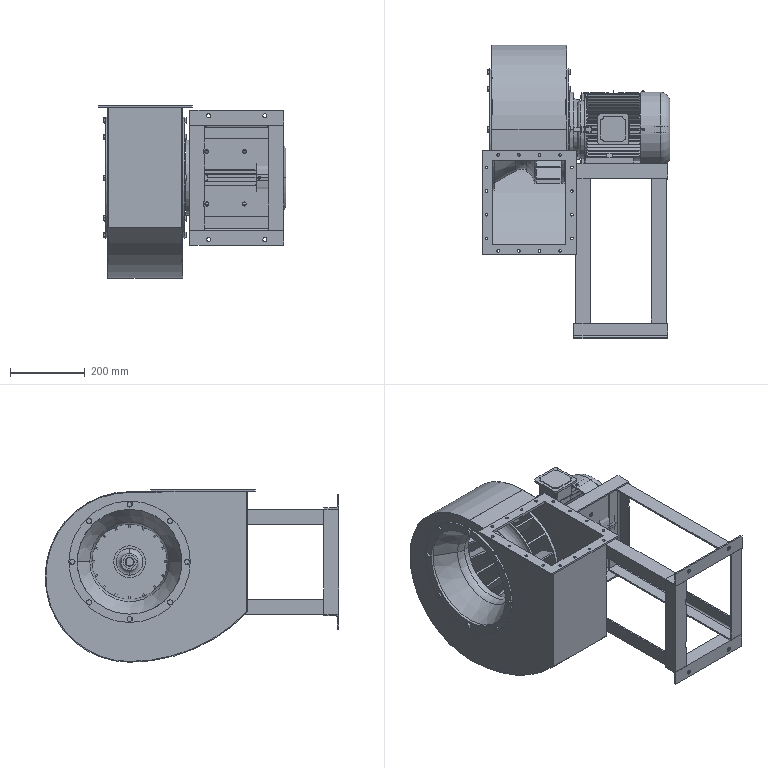Part | SolidWorks | 16 solids | 1285 faces | box 501 x 783.054 x 460 mm | volume 11094066 mm3 | plane 756 | cylinder 257 | cone 236 | torus 28 | sphere 8 | commonest cylinder face diameters 0.02 x32 7 x32 74.4 x32 10 x20 11 x16 3.937 x10